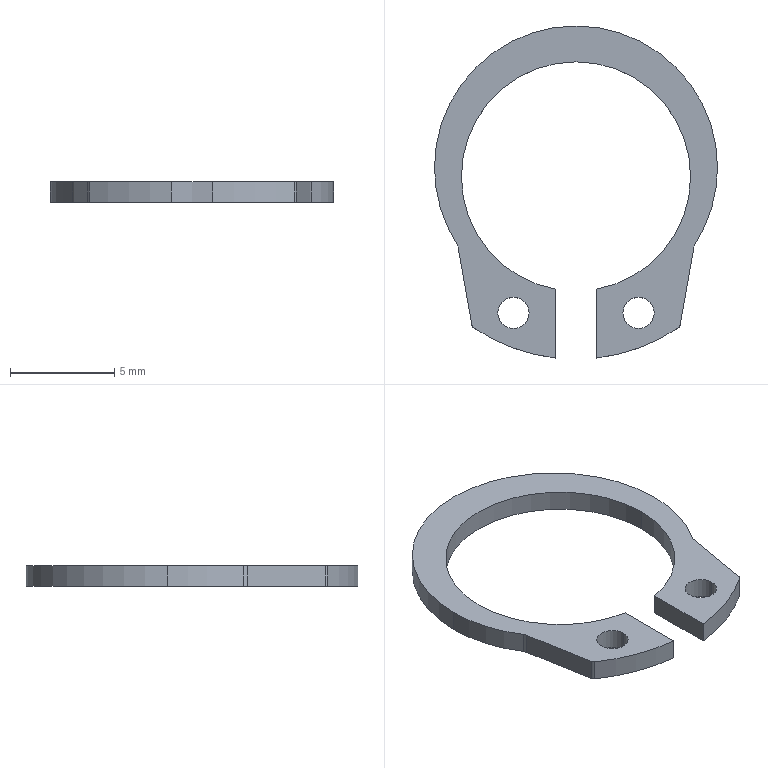Part | STEP file | 1 solid | 22 faces | box 13.58 x 15.928 x 1 mm | volume 67.493 mm3 | cylinder 16 | plane 6 | commonest cylinder face diameters 1.5 x4 11 x3 13.58 x3 0.4 x2 1 x2 17.531 x2